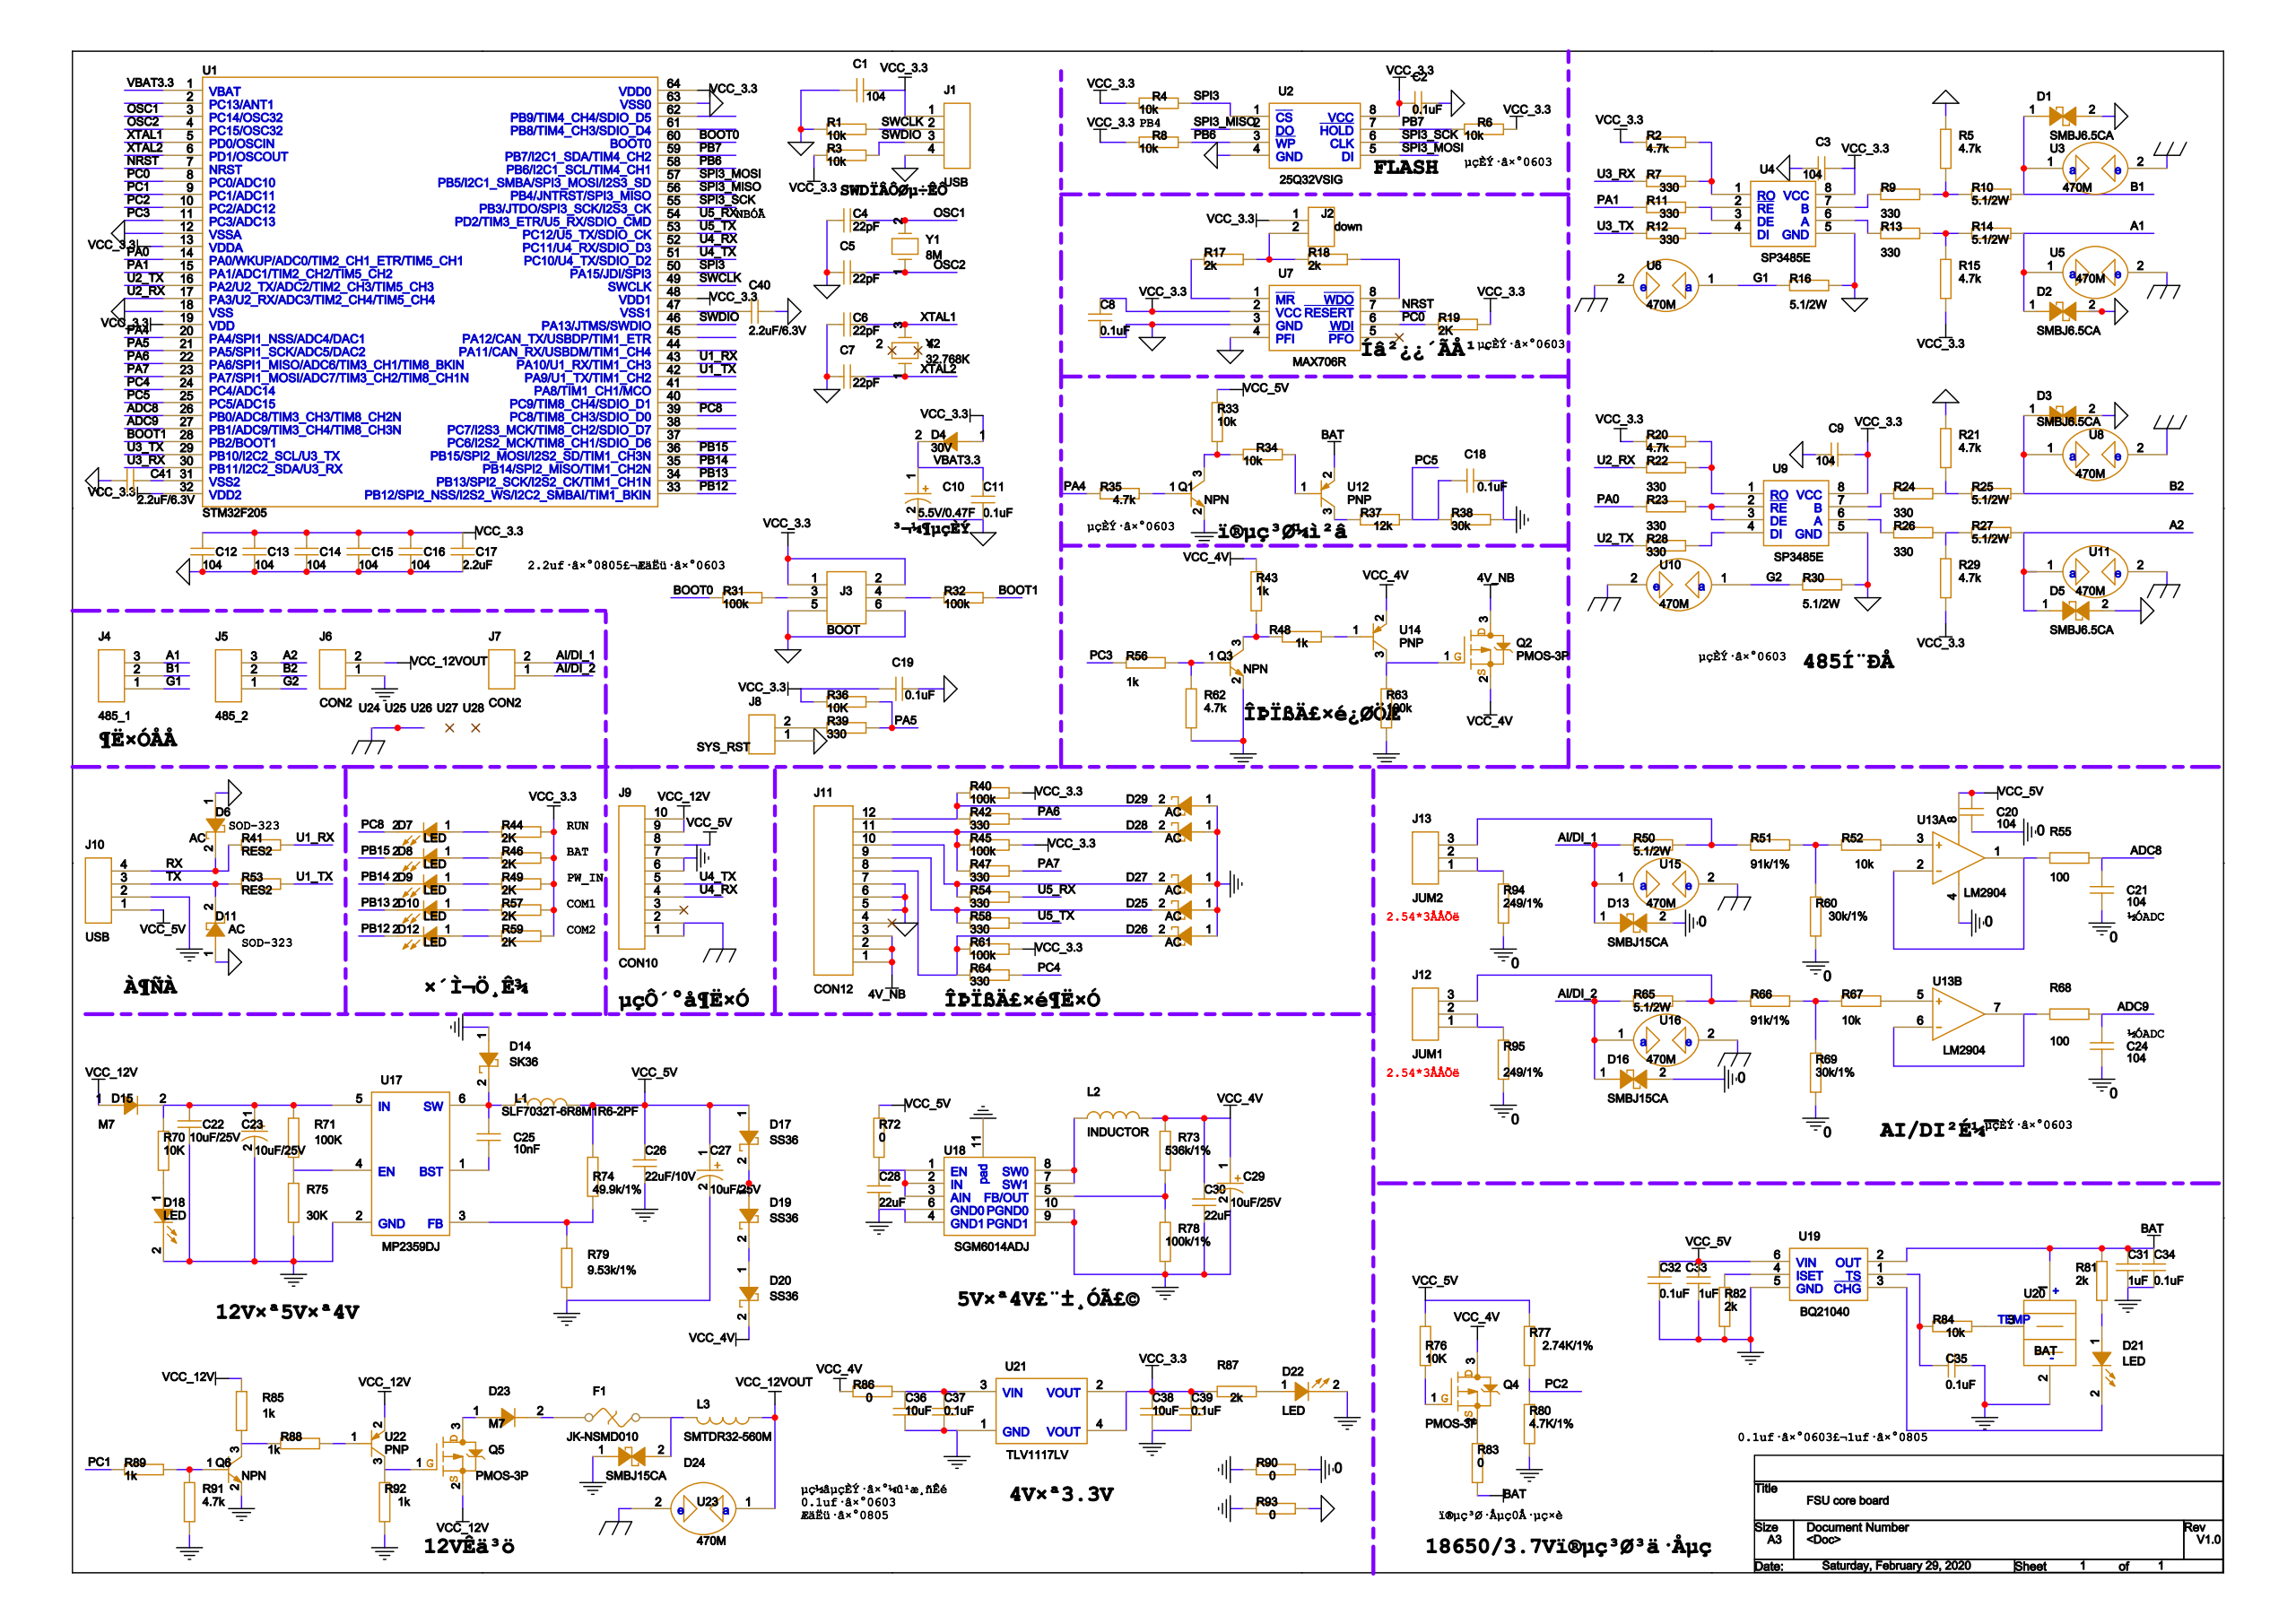Circuit board | Cadence Allegro | 216 parts | 152 nets
Bill of materials:
SYM_NAME,COMP_DEVICE_TYPE,COMP_VALUE,COMP_TOL,COMP_CLASS,REFDES
0603C,CAP NP_0603C_104,104,,IC,C1
0603C,CAP NP_0603C_0.1UF,0.1uF,,IC,C2
0603C,CAP NP_0603C_104,104,,IC,C3
0603C,CAP NP_0603C_22PF,22pF,,IC,C4
0603C,CAP NP_0603C_22PF,22pF,,IC,C5
0603C,CAP NP_0603C_22PF,22pF,,IC,C6
0603C,CAP NP_0603C_22PF,22pF,,IC,C7
0603C,CAP NP_0603C_0.1UF,0.1uF,,IC,C8
0603C,CAP NP_0603C_104,104,,IC,C9
FL,CAP POL_FL_5.5V/0.47F,5.5V/0.47F,,IC,C10
0603C,CAP NP_0603C_0.1UF,0.1uF,,IC,C11
0603C,CAP NP_0603C_104,104,,IC,C12
0603C,CAP NP_0603C_104,104,,IC,C13
0603C,CAP NP_0603C_104,104,,IC,C14
0603C,CAP NP_0603C_104,104,,IC,C15
0603C,CAP NP_0603C_104,104,,IC,C16
0805C,CAP NP_0805C_2.2UF,2.2uF,,IC,C17
0603C,CAP NP_0603C_0.1UF,0.1uF,,IC,C18
0603C,CAP NP_0603C_0.1UF,0.1uF,,IC,C19
0603C,CAP NP_0603C_104,104,,IC,C20
0603C,CAP NP_0603C_104,104,,IC,C21
0805C,CAP NP_0805C_10UF/25V,10uF/25V,,IC,C22
F80,CAP POL_F80_10UF/25V,10uF/25V,,IC,C23
0603C,CAP NP_0603C_104,104,,IC,C24
0603C,CAP NP_0603C_10NF,10nF,,IC,C25
0805C,CAP NP_0805C_22UF/10V,22uF/10V,,IC,C26
F80,CAP POL_F80_10UF/25V,10uF/25V,,IC,C27
0805C,CAP NP_0805C_22UF,22uF,,IC,C28
F80,CAP POL_F80_10UF/25V,10uF/25V,,IC,C29
0805C,CAP NP_0805C_22UF,22uF,,IC,C30
0603C,CAP NP_0603C_1UF,1uF,,IC,C31
0603C,CAP NP_0603C_0.1UF,0.1uF,,IC,C32
0603C,CAP NP_0603C_1UF,1uF,,IC,C33
0603C,CAP NP_0603C_0.1UF,0.1uF,,IC,C34
0603C,CAP NP_0603C_0.1UF,0.1uF,,IC,C35
0805C,CAP NP_0805C_10UF,10uF,,IC,C36
0603C,CAP NP_0603C_0.1UF,0.1uF,,IC,C37
0805C,CAP NP_0805C_10UF,10uF,,IC,C38
0603C,CAP NP_0603C_0.1UF,0.1uF,,IC,C39
0805C,CAP NP_0805C_2.2UF/6.3V,2.2uF/6.3V,,IC,C40
0805C,CAP NP_0805C_2.2UF/6.3V,2.2uF/6.3V,,IC,C41
SMB,DIODE-TVS_SMB_SMBJ6.5CA,SMBJ6.5CA,,IC,D1
SMB,DIODE-TVS_SMB_SMBJ6.5CA,SMBJ6.5CA,,IC,D2
SMB,DIODE-TVS_SMB_SMBJ6.5CA_1,SMBJ6.5CA,,IC,D3
SMA,DIODE_SMA_30V,30V,,IC,D4
SMB,DIODE-TVS_SMB_SMBJ6.5CA,SMBJ6.5CA,,IC,D5
SOD-323,DIODE-Z_SOD-323_AC,AC,,IC,D6
LED0603,LED_LED0603_LED,LED,,IC,D7
LED0603,LED_LED0603_LED,LED,,IC,D8
LED0603,LED_LED0603_LED,LED,,IC,D9
LED0603,LED_LED0603_LED,LED,,IC,D10
SOD-323,DIODE-Z_SOD-323_AC,AC,,IC,D11
LED0603,LED_LED0603_LED,LED,,IC,D12
SMB,DIODE-TVS_SMB_SMBJ15CA,SMBJ15CA,,IC,D13
SMA,DIODE-Z_SMA_SK36,SK36,,IC,D14
SMA,DIODE_SMA_M7,M7,,IC,D15
SMB,DIODE-TVS_SMB_SMBJ15CA,SMBJ15CA,,IC,D16
SMA,DIODE-Z_SMA_SS36,SS36,,IC,D17
LED0603,LED_LED0603_LED,LED,,IC,D18
SMA,DIODE-Z_SMA_SS36,SS36,,IC,D19
SMA,DIODE-Z_SMA_SS36,SS36,,IC,D20
LED0603,LED_LED0603_LED,LED,,IC,D21
LED0603,LED_LED0603_LED,LED,,IC,D22
SMA,DIODE_SMA_M7,M7,,IC,D23
SMB,DIODE-TVS_SMB_SMBJ15CA,SMBJ15CA,,IC,D24
SOD323,DIODE-Z_SOD323_AC,AC,,IC,D25
SOD323,DIODE-Z_SOD323_AC,AC,,IC,D26
SOD323,DIODE-Z_SOD323_AC,AC,,IC,D27
SOD323,DIODE-Z_SOD323_AC,AC,,IC,D28
SOD323,DIODE-Z_SOD323_AC,AC,,IC,D29
1206,FUSE-1_1206_JK-NSMD010,JK-NSMD010,,IC,F1
XR1X4,CON4_XR1X4_USB,USB,,IC,J1
DIP2X1,CON2_DIP2X1_DOWN,down,,IC,J2
DIP2X3,CON6A_DIP2X3_BOOT,BOOT,,IC,J3
KF2EDG-3_81-3-V,CON3_KF2EDG-3_81-3-V_485_1,485_1,,IC,J4
KF2EDG-3_81-3-V,CON3_KF2EDG-3_81-3-V_485_2,485_2,,IC,J5
KF2EDG-3_81-2-V,CON2_KF2EDG-3_81-2-V_CON2,CON2,,IC,J6
KF2EDG-3_81-2-V,CON2_KF2EDG-3_81-2-V_CON2,CON2,,IC,J7
DIP2X1,CON2_DIP2X1_SYS_RST,SYS_RST,,IC,J8
XR1X10,CON10_XR1X10_CON10,CON10,,IC,J9
XR1X4,CON4_XR1X4_USB,USB,,IC,J10
DIP1X12,CON12_DIP1X12_CON12,CON12,,IC,J11
DIP1X3,CON3_DIP1X3_JUM1,JUM1,,IC,J12
DIP1X3,CON3_DIP1X3_JUM2,JUM2,,IC,J13
6045,INDUCTOR_6045_SLF7032T-6R8M1R6-,SLF7032T-6R8M1R6-2PF,,IC,L1
6045,INDUCTOR_6045_INDUCTOR,INDUCTOR,,IC,L2
6045,INDUCTOR_6045_SMTDR32-560M,SMTDR32-560M,,IC,L3
SOT-23,NPN_SOT-23_NPN,NPN,,IC,Q1
SOT-23,PMOS-3P_SOT-23_PMOS-3P,PMOS-3P,,IC,Q2
SOT-23,NPN_SOT-23_NPN,NPN,,IC,Q3
SOT-23,PMOS-3P_SOT-23_PMOS-3P,PMOS-3P,,IC,Q4
SOT-23,PMOS-3P_SOT-23_PMOS-3P,PMOS-3P,,IC,Q5
SOT-23,NPN_SOT-23_NPN,NPN,,IC,Q6
0603R,RES2_0603R_10K,10k,,IC,R1
0603R,RES2_0603R_4.7K,4.7k,,IC,R2
0603R,RES2_0603R_10K,10k,,IC,R3
0603R,RES2_0603R_10K,10k,,IC,R4
0603R,RES2_0603R_4.7K,4.7k,,IC,R5
0603R,RES2_0603R_10K,10k,,IC,R6
0603R,RES2_0603R_330,330,,IC,R7
0603R,RES2_0603R_10K,10k,,IC,R8
0603R,RES2_0603R_330,330,,IC,R9
2512,RES2_2512_5.1/2W,5.1/2W,,IC,R10
0603R,RES2_0603R_330,330,,IC,R11
0603R,RES2_0603R_330,330,,IC,R12
0603R,RES2_0603R_330,330,,IC,R13
2512,RES2_2512_5.1/2W,5.1/2W,,IC,R14
0603R,RES2_0603R_4.7K,4.7k,,IC,R15
2512,RES2_2512_5.1/2W,5.1/2W,,IC,R16
0603R,RES2_0603R_2K,2k,,IC,R17
0603R,RES2_0603R_2K,2k,,IC,R18
0603R,RES2_0603R_2K,2k,,IC,R19
0603R,RES2_0603R_4.7K,4.7k,,IC,R20
0603R,RES2_0603R_4.7K,4.7k,,IC,R21
0603R,RES2_0603R_330,330,,IC,R22
0603R,RES2_0603R_330,330,,IC,R23
0603R,RES2_0603R_330,330,,IC,R24
2512,RES2_2512_5.1/2W,5.1/2W,,IC,R25
0603R,RES2_0603R_330,330,,IC,R26
2512,RES2_2512_5.1/2W,5.1/2W,,IC,R27
0603R,RES2_0603R_330,330,,IC,R28
0603R,RES2_0603R_4.7K,4.7k,,IC,R29
2512,RES2_2512_5.1/2W,5.1/2W,,IC,R30
0603R,RES2_0603R_100K,100k,,IC,R31
0603R,RES2_0603R_100K,100k,,IC,R32
0603R,RES2_0603R_10K,10k,,IC,R33
0603R,RES2_0603R_10K,10k,,IC,R34
0603R,RES2_0603R_4.7K,4.7k,,IC,R35
0603R,RES2_0603R_10K,10k,,IC,R36
0603R,RES2_0603R_12K,12k,,IC,R37
0603R,RES2_0603R_30K,30k,,IC,R38
0603R,RES2_0603R_330,330,,IC,R39
0603R,RES2_0603R_100K,100k,,IC,R40
0603R,RES2_0603R_RES2,RES2,,IC,R41
0603R,RES2_0603R_330,330,,IC,R42
0603R,RES2_0603R_1K,1k,,IC,R43
0603R,RES2_0603R_2K,2k,,IC,R44
0603R,RES2_0603R_100K,100k,,IC,R45
0603R,RES2_0603R_2K,2k,,IC,R46
0603R,RES2_0603R_330,330,,IC,R47
0603R,RES2_0603R_1K,1k,,IC,R48
0603R,RES2_0603R_2K,2k,,IC,R49
2512,RES2_2512_5.1/2W,5.1/2W,,IC,R50
0603R,RES2_0603R_91K/1%,91k/1%,,IC,R51
0603R,RES2_0603R_10K,10k,,IC,R52
0603R,RES2_0603R_RES2,RES2,,IC,R53
0603R,RES2_0603R_330,330,,IC,R54
0603R,RES2_0603R_100,100,,IC,R55
0603R,RES2_0603R_1K,1k,,IC,R56
0603R,RES2_0603R_2K,2k,,IC,R57
0603R,RES2_0603R_330,330,,IC,R58
0603R,RES2_0603R_2K,2k,,IC,R59
0603R,RES2_0603R_30K/1%,30k/1%,,IC,R60
0603R,RES2_0603R_100K,100k,,IC,R61
0603R,RES2_0603R_4.7K,4.7k,,IC,R62
0603R,RES2_0603R_100K,100k,,IC,R63
0603R,RES2_0603R_330,330,,IC,R64
2512,RES2_2512_5.1/2W,5.1/2W,,IC,R65
0603R,RES2_0603R_91K/1%,91k/1%,,IC,R66
0603R,RES2_0603R_10K,10k,,IC,R67
0603R,RES2_0603R_100,100,,IC,R68
0603R,RES2_0603R_30K/1%,30k/1%,,IC,R69
0603R,RES2_0603R_10K,10k,,IC,R70
0603R,RES2_0603R_100K,100k,,IC,R71
0603R,RES2_0603R_0,0,,IC,R72
0603R,RES2_0603R_536K/1%,536k/1%,,IC,R73
0603R,RES2_0603R_49.9K/1%,49.9k/1%,,IC,R74
0603R,RES2_0603R_30K,30k,,IC,R75
0603R,RES2_0603R_10K,10k,,IC,R76
0603R,RES2_0603R_2.74K/1%,2.74K/1%,,IC,R77
0603R,RES2_0603R_100K/1%,100k/1%,,IC,R78
0603R,RES2_0603R_9.53K/1%,9.53k/1%,,IC,R79
0603R,RES2_0603R_4.7K/1%,4.7K/1%,,IC,R80
0603R,RES2_0603R_2K,2k,,IC,R81
0603R,RES2_0603R_2K,2k,,IC,R82
0603R,RES2_0603R_0,0,,IC,R83
0603R,RES2_0603R_10K,10k,,IC,R84
0603R,RES2_0603R_1K,1k,,IC,R85
0603R,RES2_0603R_0,0,,IC,R86
0603R,RES2_0603R_2K,2k,,IC,R87
0603R,RES2_0603R_1K,1k,,IC,R88
0603R,RES2_0603R_1K,1k,,IC,R89
0603R,RES2_0603R_0,0,,IC,R90
0603R,RES2_0603R_4.7K,4.7k,,IC,R91
0603R,RES2_0603R_1K,1k,,IC,R92
0603R,RES2_0603R_0,0,,IC,R93
0603R,RES2_0603R_249/1%,249/1%,,IC,R94
0603R,RES2_0603R_249/1%,249/1%,,IC,R95
LQFP-64,205RGT6_0_LQFP-64_STM32F205,STM32F205,,IC,U1
SOIC-8_208,W25Q32_SOIC-8_208_25Q32VSIG,25Q32VSIG,,IC,U2
SMD5050,GDT_SMD5050_470M,470M,,IC,U3
SO8,SP485EE_SO8_SP3485E,SP3485E,,IC,U4
SMD5050,GDT_SMD5050_470M,470M,,IC,U5
SMD5050,GDT_SMD5050_470M,470M,,IC,U6
SO8,MAX706R_SO8_MAX706R,MAX706R,,IC,U7
SMD5050,GDT_SMD5050_470M,470M,,IC,U8
SO8,SP485EE_SO8_SP3485E,SP3485E,,IC,U9
SMD5050,GDT_SMD5050_470M,470M,,IC,U10
SMD5050,GDT_SMD5050_470M,470M,,IC,U11
SOT-23,PNP_SOT-23_PNP,PNP,,IC,U12
SO8,LM358_SO8_LM2904,LM2904,,IC,U13
SOT-23,PNP_SOT-23_PNP,PNP,,IC,U14
SMD5050,GDT_SMD5050_470M,470M,,IC,U15
SMD5050,GDT_SMD5050_470M,470M,,IC,U16
SOT23-6,MP2359DJ_SOT23-6_MP2359DJ,MP2359DJ,,IC,U17
TDFN-3X3-10L,SGM6014_ADJ_1_TDFN-3X3-10L_SGM6,SGM6014ADJ,,IC,U18
SOT23-6,BQ21040_SOT23-6_BQ21040,BQ21040,,IC,U19
XR1X3,BATTERT_XR1X3_BAT,BAT,,IC,U20
SOT-223,TLV1117LV_SOT-223_TLV1117LV,TLV1117LV,,IC,U21
SOT-23,PNP_SOT-23_PNP,PNP,,IC,U22
SMD5050,GDT_SMD5050_470M,470M,,IC,U23
HOLE,TEST POINT A_HOLE_TEST POINT A,TEST POINT A,,IC,U24
HOLE,TEST POINT A_HOLE_TEST POINT A,TEST POINT A,,IC,U25
HOLE,TEST POINT A_HOLE_TEST POINT A,TEST POINT A,,IC,U26
HOLE,TEST POINT A_HOLE_TEST POINT A,TEST POINT A,,IC,U27
HOLE,TEST POINT A_HOLE_TEST POINT A,TEST POINT A,,IC,U28
XTAL3215,CRYSTAL_XTAL3215_8M,8M,,IC,Y1
XTAL3225,CRYSTAL_0_XTAL3225_32.768K,32.768K,,IC,Y2
Netlist (net: part-pin ...):
VCC_4V: C29-1 C30-1 D20-2 L2-2 Q2-2 Q4-3 R43-2 R73-1 R86-1 U14-2
N42321: Q2-1 R63-2 U14-3
4V_NB: J11-1 J11-2 J11-3 Q2-3
N66169: Q4-1 R76-1
N667041: Q4-2 R83-2
VCC_12V: D15-1 J9-9 J9-10 Q5-2 R85-2 U22-2
N48219: Q5-1 R92-2 U22-3
N278477: D23-1 Q5-3
N54158: C36-2 C37-2 R86-2 U21-3
GND_POWER: C18-2 C22-2 C23-2 C26-2 C27-2 C28-2 C29-2 C30-2 C31-2 C32-2 C33-2 C34-2 C35-2 C36-1 C37-1 C38-1 C39-1 D14-1 D18-2 D22-2 D24-1 D25-1 D26-1 D27-1 D28-1 D29-1 J6-1 J9-6 J9-7 J10-2 Q1-2 Q3-2 Q6-2 R38-2 R62-2 R63-1 R75-1 R78-2 R79-1 R80-1 R82-2 R90-1 R91-1 R92-1 R93-1 U17-2 U18-4 U18-6 U18-9 U18-10 U18-11 U19-5 U20-2 U21-1
VCC_3.3: C1-1 C2-1 C3-2 C8-1 C9-2 C12-1 C13-1 C14-1 C15-1 C16-1 C17-1 C19-2 C38-2 C39-2 D4-1 J1-1 J2-1 J3-1 J3-2 R2-2 R3-1 R4-1 R6-2 R8-1 R15-2 R19-2 R20-2 R29-2 R36-2 R40-2 R44-2 R45-2 R46-2 R49-2 R57-2 R59-2 R61-2 R87-1 U1-13 U1-19 U1-32 U1-48 U1-64 U2-8 U4-8 U7-2 U9-8 U21-2 U21-4
N08828: C22-1 C23-1 D15-2 R70-2 R71-2 U17-5
GND_SIGNAL: C1-2 C2-2 C3-1 C4-2 C5-2 C6-2 C7-2 C8-2 C9-1 C10-2 C11-2 C12-2 C13-2 C14-2 C15-2 C16-2 C17-2 C19-1 C40-2 C41-1 D1-2 D2-2 D3-2 D5-2 D6-1 D11-1 J1-4 J3-5 J3-6 J8-1 J11-5 J11-6 J11-7 R1-1 R5-1 R16-1 R21-1 R30-1 R93-2 U1-12 U1-18 U1-63 U2-4 U4-5 U7-3 U7-4 U9-5
G1: J4-1 R16-2 U6-1
G2: J5-1 R30-2 U10-1
N22081: R5-2 R9-2 R10-1
B1: D1-1 J4-2 R10-2 U3-1
N22085: R13-2 R14-1 R15-1
A1: D2-1 J4-3 R14-2 U5-1
N27071: R21-2 R24-2 R25-1
B2: D3-1 J5-2 R25-2 U8-1
N27075: R26-2 R27-1 R29-1
A2: D5-1 J5-3 R27-2 U11-1
AI/DI_1: D13-1 J7-2 R50-1 U15-1
N139834: J13-3 R50-2 R51-1
AI/DI_2: D16-1 J7-1 R65-1 U16-1
N139830: J12-3 R65-2 R66-2
N09349: C25-1 D14-2 L1-1 U17-6
VCC_5V: C20-1 C26-1 C27-1 C32-1 C33-1 D17-1 J9-8 J10-1 L1-2 R33-2 R72-2 R74-1 R76-2 R77-2 U13-8 U19-6
N36959: L2-1 U18-7 U18-8
VCC_12VOUT: J6-2 L3-1 U23-1
N49209: D24-2 F1-1 L3-2
GND_EARTH: J9-1 J9-2 U3-2 U5-2 U6-2 U8-2 U10-2 U11-2 U15-2 U16-2 U23-2 U24-1 U25-1 U26-1
N243486: C40-1 U1-47
N243888: C41-2 U1-31
N36926: C28-1 R72-1 U18-1 U18-2 U18-3
N36943: R73-2 R78-1 U18-5
N81110: J2-2 R17-2 R18-1
N217417: J12-1 J12-2 R95-2
N217431: J13-1 J13-2 R94-2
N92407: J3-3 R31-2
N92258: J3-4 R32-1
SWCLK: J1-2 R1-2 U1-49
SWDIO: J1-3 R3-2 U1-46
TX: D11-2 J10-3 R53-1
RX: D6-2 J10-4 R41-1
U4_RX: J9-4 U1-52
U4_TX: J9-5 U1-51
BAT: C31-1 C34-1 R81-1 R83-1 U12-2 U19-2 U20-1
N386422: R84-2 U20-3
VBAT3.3: C10-1 C11-1 D4-2 U1-1
N94594: D25-2 J11-9 R58-1
N94660: D26-2 J11-8 R61-1 R64-1
N94590: D27-2 J11-10 R54-1
N130990: D28-2 J11-11 R45-1 R47-1
N93753: D29-2 J11-12 R40-1 R42-1
N48673: D23-2 F1-2
0: C20-2 C21-2 C24-2 D13-2 D16-2 R60-1 R69-2 R90-2 R94-1 R95-1 U13-4
N810071: J8-2 R39-1
ADC8: C21-1 R55-1 U1-26
ADC9: C24-1 R68-2 U1-27
PC5: C18-1 R37-2 R38-1 U1-25
N41072: C35-1 R84-1 U19-1
N09345: C25-2 U17-1
OSC1: C4-1 U1-3 Y1-2
OSC2: C5-1 U1-4 Y1-1
XTAL1: C6-1 U1-5 Y2-3
XTAL2: C7-1 U1-6 Y2-1
N44275: D10-1 R57-1
PB13: D10-2 U1-34
N44279: D12-1 R59-1
PB12: D12-2 U1-33
N458610: D18-1 R70-1
N38563: D21-1 R81-2
N38355: D21-2 U19-3
N550141: D22-1 R87-2
N44251: D7-1 R44-1
PC8: D7-2 U1-39
N44255: D8-1 R46-1
PB15: D8-2 U1-36
N44271: D9-1 R49-1
PB14: D9-2 U1-35
N29354: D17-2 D19-1
N159349: D19-2 D20-1
N43531: Q1-1 R35-2
N70368: Q1-3 R33-1 R34-2
N42077: Q3-3 R43-1 R48-1
N42054: Q3-1 R56-2 R62-1
N48164: Q6-3 R85-1 R88-1
N47266: Q6-1 R89-2 R91-2
N43395: R34-1 U12-1
PA5: R36-1 R39-2 U1-21
SPI3: R4-2 U1-50 U2-1
N30746: R51-2 R52-1 R60-2
N303440: R52-2 U13-3
PB7: R6-1 U1-59 U2-7
N303730: R67-1 U13-5
N30755: R66-1 R67-2 R69-1
PB6: R8-2 U1-58 U2-3
PA1: R11-1 U1-15
N10035: R11-2 U4-2 U4-3
U3_TX: R12-1 U1-29
N21958: R12-2 U4-4
N22072: R13-1 U4-6
U2_RX: R22-1 U1-17
N26999: R20-1 R22-2 U9-1
PA0: R23-1 U1-14
N27319: R23-2 U9-2 U9-3
N27015: R24-1 U9-7
N27019: R26-1 U9-6
U2_TX: R28-1 U1-16
N27011: R28-2 U9-4
PA6: R42-2 U1-22
PA7: R47-2 U1-23
U5_RX: R54-2 U1-54
U5_TX: R58-2 U1-53
PC4: R64-2 U1-24
U3_RX: R7-1 U1-30
N21940: R2-1 R7-2 U4-1
N22000: R9-1 U4-7
PA4: R35-1 U1-20
N80858: R17-1 U7-1
N81178: R18-2 U7-8
PC0: R19-1 U1-8 U7-6
N37896: R82-1 U19-4
BOOT0: R31-1 U1-60
BOOT1: R32-2 U1-28
N08824: R71-1 R75-2 U17-4
N43391: R37-1 U12-3
U1_RX: R41-2 U1-43
U1_TX: R53-2 U1-42
N42317: R48-2 U14-1
PC3: R56-1 U1-11
N48169: R88-2 U22-1
PC1: R89-1 U1-9
N30779: R55-2 U13-1 U13-2
N30764: R68-1 U13-6 U13-7
N09119: R74-2 R79-2 U17-3
PC2: R77-1 R80-2 U1-10
NRST: U1-7 U7-7
N45595: U1-44
N45591: U1-45
N45695: U1-41
SPI3_SCK: U1-55 U2-6
SPI3_MISO: U1-56 U2-2
SPI3_MOSI: U1-57 U2-5
N45439: U1-61
N45435: U1-62
N44943: U1-2
N123538: U1-37
N45707: U1-38
N45699: U1-40